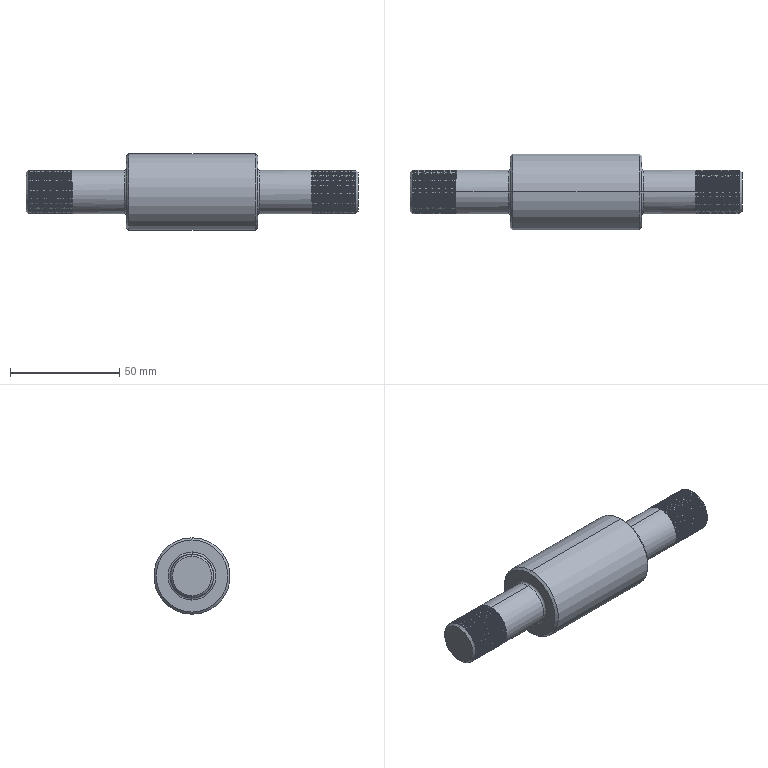Part | STEP file | Hydraulic cylinder hinge pin stepped shaft | 1 solid | 232 faces | box 152 x 35 x 35 mm | volume 86130 mm3 | cylinder 206 | cone 8 | plane 8 | spline 6 | torus 4 | commonest cylinder face diameters 20 x204 35 x2